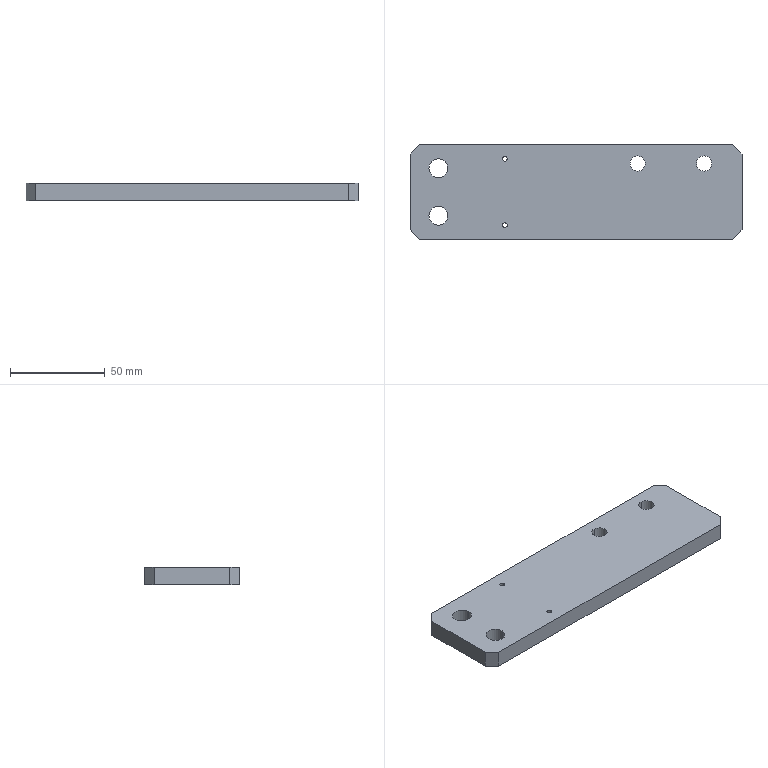Part | STEP file | J013-EBZ05-26-06-Part-1 | 1 solid | 22 faces | box 175 x 50 x 9 mm | volume 75893 mm3 | cylinder 12 | plane 10 | commonest cylinder face diameters 2.5 x4 8 x4 10 x4
STEP:
#1=CARTESIAN_POINT('',(51.25,42.5,9.));
#2=VERTEX_POINT('',#1);
#3=CARTESIAN_POINT('',(48.75,42.5,9.));
#4=VERTEX_POINT('',#3);
#5=CARTESIAN_POINT('',(50.,42.5,9.));
#6=DIRECTION('',(0.,0.,-1.));
#7=DIRECTION('',(-1.,0.,0.));
#8=AXIS2_PLACEMENT_3D('',#5,#6,#7);
#9=CIRCLE('',#8,1.25);
#10=EDGE_CURVE('',#2,#4,#9,.T.);
#11=ORIENTED_EDGE('',*,*,#10,.F.);
#12=CARTESIAN_POINT('',(51.25,42.5,0.));
#13=VERTEX_POINT('',#12);
#14=CARTESIAN_POINT('',(51.25,42.5,9.));
#15=DIRECTION('',(0.,0.,-1.));
#16=VECTOR('',#15,1000.);
#17=LINE('',#14,#16);
#18=EDGE_CURVE('',#2,#13,#17,.T.);
#19=ORIENTED_EDGE('',*,*,#18,.T.);
#20=CARTESIAN_POINT('',(48.75,42.5,0.));
#21=VERTEX_POINT('',#20);
#22=CARTESIAN_POINT('',(50.,42.5,0.));
#23=DIRECTION('',(0.,0.,1.));
#24=DIRECTION('',(1.,0.,0.));
#25=AXIS2_PLACEMENT_3D('',#22,#23,#24);
#26=CIRCLE('',#25,1.25);
#27=EDGE_CURVE('',#21,#13,#26,.T.);
#28=ORIENTED_EDGE('',*,*,#27,.F.);
#29=CARTESIAN_POINT('',(48.75,42.5,9.));
#30=DIRECTION('',(0.,0.,-1.));
#31=VECTOR('',#30,1000.);
#32=LINE('',#29,#31);
#33=EDGE_CURVE('',#4,#21,#32,.T.);
#34=ORIENTED_EDGE('',*,*,#33,.F.);
#35=EDGE_LOOP('',(#11,#19,#28,#34));
#36=FACE_OUTER_BOUND('',#35,.T.);
#37=CARTESIAN_POINT('',(50.,42.5,9.));
#38=DIRECTION('',(0.,0.,-1.));
#39=DIRECTION('',(-1.,0.,0.));
#40=AXIS2_PLACEMENT_3D('',#37,#38,#39);
#41=CYLINDRICAL_SURFACE('',#40,1.25);
#42=ADVANCED_FACE('',(#36),#41,.F.);
#43=CARTESIAN_POINT('',(50.,6.25,9.));
#44=VERTEX_POINT('',#43);
#45=CARTESIAN_POINT('',(50.,8.75,9.));
#46=VERTEX_POINT('',#45);
#47=CARTESIAN_POINT('',(50.,7.5,9.));
#48=DIRECTION('',(0.,0.,-1.));
#49=DIRECTION('',(0.,1.,0.));
#50=AXIS2_PLACEMENT_3D('',#47,#48,#49);
#51=CIRCLE('',#50,1.25);
#52=EDGE_CURVE('',#44,#46,#51,.T.);
#53=ORIENTED_EDGE('',*,*,#52,.F.);
#54=CARTESIAN_POINT('',(50.,6.25,0.));
#55=VERTEX_POINT('',#54);
#56=CARTESIAN_POINT('',(50.,6.25,9.));
#57=DIRECTION('',(0.,0.,-1.));
#58=VECTOR('',#57,1000.);
#59=LINE('',#56,#58);
#60=EDGE_CURVE('',#44,#55,#59,.T.);
#61=ORIENTED_EDGE('',*,*,#60,.T.);
#62=CARTESIAN_POINT('',(50.,8.75,0.));
#63=VERTEX_POINT('',#62);
#64=CARTESIAN_POINT('',(50.,7.5,0.));
#65=DIRECTION('',(0.,0.,1.));
#66=DIRECTION('',(0.,-1.,0.));
#67=AXIS2_PLACEMENT_3D('',#64,#65,#66);
#68=CIRCLE('',#67,1.25);
#69=EDGE_CURVE('',#63,#55,#68,.T.);
#70=ORIENTED_EDGE('',*,*,#69,.F.);
#71=CARTESIAN_POINT('',(50.,8.75,9.));
#72=DIRECTION('',(0.,0.,-1.));
#73=VECTOR('',#72,1000.);
#74=LINE('',#71,#73);
#75=EDGE_CURVE('',#46,#63,#74,.T.);
#76=ORIENTED_EDGE('',*,*,#75,.F.);
#77=EDGE_LOOP('',(#53,#61,#70,#76));
#78=FACE_OUTER_BOUND('',#77,.T.);
#79=CARTESIAN_POINT('',(50.,7.5,9.));
#80=DIRECTION('',(0.,0.,-1.));
#81=DIRECTION('',(0.,1.,0.));
#82=AXIS2_PLACEMENT_3D('',#79,#80,#81);
#83=CYLINDRICAL_SURFACE('',#82,1.25);
#84=ADVANCED_FACE('',(#78),#83,.F.);
#85=CARTESIAN_POINT('',(155.,36.,9.));
#86=VERTEX_POINT('',#85);
#87=CARTESIAN_POINT('',(155.,44.,9.));
#88=VERTEX_POINT('',#87);
#89=CARTESIAN_POINT('',(155.,40.,9.));
#90=DIRECTION('',(0.,0.,-1.));
#91=DIRECTION('',(0.,1.,0.));
#92=AXIS2_PLACEMENT_3D('',#89,#90,#91);
#93=CIRCLE('',#92,4.);
#94=EDGE_CURVE('',#86,#88,#93,.T.);
#95=ORIENTED_EDGE('',*,*,#94,.F.);
#96=CARTESIAN_POINT('',(155.,36.,0.));
#97=VERTEX_POINT('',#96);
#98=CARTESIAN_POINT('',(155.,36.,9.));
#99=DIRECTION('',(0.,0.,-1.));
#100=VECTOR('',#99,1000.);
#101=LINE('',#98,#100);
#102=EDGE_CURVE('',#86,#97,#101,.T.);
#103=ORIENTED_EDGE('',*,*,#102,.T.);
#104=CARTESIAN_POINT('',(155.,44.,0.));
#105=VERTEX_POINT('',#104);
#106=CARTESIAN_POINT('',(155.,40.,0.));
#107=DIRECTION('',(0.,0.,1.));
#108=DIRECTION('',(0.,-1.,0.));
#109=AXIS2_PLACEMENT_3D('',#106,#107,#108);
#110=CIRCLE('',#109,4.);
#111=EDGE_CURVE('',#105,#97,#110,.T.);
#112=ORIENTED_EDGE('',*,*,#111,.F.);
#113=CARTESIAN_POINT('',(155.,44.,9.));
#114=DIRECTION('',(0.,0.,-1.));
#115=VECTOR('',#114,1000.);
#116=LINE('',#113,#115);
#117=EDGE_CURVE('',#88,#105,#116,.T.);
#118=ORIENTED_EDGE('',*,*,#117,.F.);
#119=EDGE_LOOP('',(#95,#103,#112,#118));
#120=FACE_OUTER_BOUND('',#119,.T.);
#121=CARTESIAN_POINT('',(155.,40.,9.));
#122=DIRECTION('',(0.,0.,-1.));
#123=DIRECTION('',(0.,1.,0.));
#124=AXIS2_PLACEMENT_3D('',#121,#122,#123);
#125=CYLINDRICAL_SURFACE('',#124,4.);
#126=ADVANCED_FACE('',(#120),#125,.F.);
#127=CARTESIAN_POINT('',(120.,36.,9.));
#128=VERTEX_POINT('',#127);
#129=CARTESIAN_POINT('',(120.,44.,9.));
#130=VERTEX_POINT('',#129);
#131=CARTESIAN_POINT('',(120.,40.,9.));
#132=DIRECTION('',(0.,0.,-1.));
#133=DIRECTION('',(0.,1.,0.));
#134=AXIS2_PLACEMENT_3D('',#131,#132,#133);
#135=CIRCLE('',#134,4.);
#136=EDGE_CURVE('',#128,#130,#135,.T.);
#137=ORIENTED_EDGE('',*,*,#136,.F.);
#138=CARTESIAN_POINT('',(120.,36.,0.));
#139=VERTEX_POINT('',#138);
#140=CARTESIAN_POINT('',(120.,36.,9.));
#141=DIRECTION('',(0.,0.,-1.));
#142=VECTOR('',#141,1000.);
#143=LINE('',#140,#142);
#144=EDGE_CURVE('',#128,#139,#143,.T.);
#145=ORIENTED_EDGE('',*,*,#144,.T.);
#146=CARTESIAN_POINT('',(120.,44.,0.));
#147=VERTEX_POINT('',#146);
#148=CARTESIAN_POINT('',(120.,40.,0.));
#149=DIRECTION('',(0.,0.,1.));
#150=DIRECTION('',(0.,-1.,0.));
#151=AXIS2_PLACEMENT_3D('',#148,#149,#150);
#152=CIRCLE('',#151,4.);
#153=EDGE_CURVE('',#147,#139,#152,.T.);
#154=ORIENTED_EDGE('',*,*,#153,.F.);
#155=CARTESIAN_POINT('',(120.,44.,9.));
#156=DIRECTION('',(0.,0.,-1.));
#157=VECTOR('',#156,1000.);
#158=LINE('',#155,#157);
#159=EDGE_CURVE('',#130,#147,#158,.T.);
#160=ORIENTED_EDGE('',*,*,#159,.F.);
#161=EDGE_LOOP('',(#137,#145,#154,#160));
#162=FACE_OUTER_BOUND('',#161,.T.);
#163=CARTESIAN_POINT('',(120.,40.,9.));
#164=DIRECTION('',(0.,0.,-1.));
#165=DIRECTION('',(0.,1.,0.));
#166=AXIS2_PLACEMENT_3D('',#163,#164,#165);
#167=CYLINDRICAL_SURFACE('',#166,4.);
#168=ADVANCED_FACE('',(#162),#167,.F.);
#169=CARTESIAN_POINT('',(20.,37.5,9.));
#170=VERTEX_POINT('',#169);
#171=CARTESIAN_POINT('',(10.,37.5,9.));
#172=VERTEX_POINT('',#171);
#173=CARTESIAN_POINT('',(15.,37.5,9.));
#174=DIRECTION('',(0.,0.,-1.));
#175=DIRECTION('',(-1.,0.,0.));
#176=AXIS2_PLACEMENT_3D('',#173,#174,#175);
#177=CIRCLE('',#176,5.);
#178=EDGE_CURVE('',#170,#172,#177,.T.);
#179=ORIENTED_EDGE('',*,*,#178,.F.);
#180=CARTESIAN_POINT('',(20.,37.5,0.));
#181=VERTEX_POINT('',#180);
#182=CARTESIAN_POINT('',(20.,37.5,9.));
#183=DIRECTION('',(0.,0.,-1.));
#184=VECTOR('',#183,1000.);
#185=LINE('',#182,#184);
#186=EDGE_CURVE('',#170,#181,#185,.T.);
#187=ORIENTED_EDGE('',*,*,#186,.T.);
#188=CARTESIAN_POINT('',(10.,37.5,0.));
#189=VERTEX_POINT('',#188);
#190=CARTESIAN_POINT('',(15.,37.5,0.));
#191=DIRECTION('',(0.,0.,1.));
#192=DIRECTION('',(1.,0.,0.));
#193=AXIS2_PLACEMENT_3D('',#190,#191,#192);
#194=CIRCLE('',#193,5.);
#195=EDGE_CURVE('',#189,#181,#194,.T.);
#196=ORIENTED_EDGE('',*,*,#195,.F.);
#197=CARTESIAN_POINT('',(10.,37.5,9.));
#198=DIRECTION('',(0.,0.,-1.));
#199=VECTOR('',#198,1000.);
#200=LINE('',#197,#199);
#201=EDGE_CURVE('',#172,#189,#200,.T.);
#202=ORIENTED_EDGE('',*,*,#201,.F.);
#203=EDGE_LOOP('',(#179,#187,#196,#202));
#204=FACE_OUTER_BOUND('',#203,.T.);
#205=CARTESIAN_POINT('',(15.,37.5,9.));
#206=DIRECTION('',(0.,0.,-1.));
#207=DIRECTION('',(-1.,0.,0.));
#208=AXIS2_PLACEMENT_3D('',#205,#206,#207);
#209=CYLINDRICAL_SURFACE('',#208,5.);
#210=ADVANCED_FACE('',(#204),#209,.F.);
#211=CARTESIAN_POINT('',(20.,12.5,9.));
#212=VERTEX_POINT('',#211);
#213=CARTESIAN_POINT('',(10.,12.5,9.));
#214=VERTEX_POINT('',#213);
#215=CARTESIAN_POINT('',(15.,12.5,9.));
#216=DIRECTION('',(0.,0.,-1.));
#217=DIRECTION('',(-1.,0.,0.));
#218=AXIS2_PLACEMENT_3D('',#215,#216,#217);
#219=CIRCLE('',#218,5.);
#220=EDGE_CURVE('',#212,#214,#219,.T.);
#221=ORIENTED_EDGE('',*,*,#220,.F.);
#222=CARTESIAN_POINT('',(20.,12.5,0.));
#223=VERTEX_POINT('',#222);
#224=CARTESIAN_POINT('',(20.,12.5,9.));
#225=DIRECTION('',(0.,0.,-1.));
#226=VECTOR('',#225,1000.);
#227=LINE('',#224,#226);
#228=EDGE_CURVE('',#212,#223,#227,.T.);
#229=ORIENTED_EDGE('',*,*,#228,.T.);
#230=CARTESIAN_POINT('',(10.,12.5,0.));
#231=VERTEX_POINT('',#230);
#232=CARTESIAN_POINT('',(15.,12.5,0.));
#233=DIRECTION('',(0.,0.,1.));
#234=DIRECTION('',(1.,0.,0.));
#235=AXIS2_PLACEMENT_3D('',#232,#233,#234);
#236=CIRCLE('',#235,5.);
#237=EDGE_CURVE('',#231,#223,#236,.T.);
#238=ORIENTED_EDGE('',*,*,#237,.F.);
#239=CARTESIAN_POINT('',(10.,12.5,9.));
#240=DIRECTION('',(0.,0.,-1.));
#241=VECTOR('',#240,1000.);
#242=LINE('',#239,#241);
#243=EDGE_CURVE('',#214,#231,#242,.T.);
#244=ORIENTED_EDGE('',*,*,#243,.F.);
#245=EDGE_LOOP('',(#221,#229,#238,#244));
#246=FACE_OUTER_BOUND('',#245,.T.);
#247=CARTESIAN_POINT('',(15.,12.5,9.));
#248=DIRECTION('',(0.,0.,-1.));
#249=DIRECTION('',(-1.,0.,0.));
#250=AXIS2_PLACEMENT_3D('',#247,#248,#249);
#251=CYLINDRICAL_SURFACE('',#250,5.);
#252=ADVANCED_FACE('',(#246),#251,.F.);
#253=ORIENTED_EDGE('',*,*,#27,.T.);
#254=CARTESIAN_POINT('',(50.,42.5,0.));
#255=DIRECTION('',(0.,0.,1.));
#256=DIRECTION('',(1.,0.,0.));
#257=AXIS2_PLACEMENT_3D('',#254,#255,#256);
#258=CIRCLE('',#257,1.25);
#259=EDGE_CURVE('',#13,#21,#258,.T.);
#260=ORIENTED_EDGE('',*,*,#259,.T.);
#261=EDGE_LOOP('',(#253,#260));
#262=FACE_BOUND('',#261,.T.);
#263=ORIENTED_EDGE('',*,*,#69,.T.);
#264=CARTESIAN_POINT('',(50.,7.5,0.));
#265=DIRECTION('',(0.,0.,1.));
#266=DIRECTION('',(0.,-1.,0.));
#267=AXIS2_PLACEMENT_3D('',#264,#265,#266);
#268=CIRCLE('',#267,1.25);
#269=EDGE_CURVE('',#55,#63,#268,.T.);
#270=ORIENTED_EDGE('',*,*,#269,.T.);
#271=EDGE_LOOP('',(#263,#270));
#272=FACE_BOUND('',#271,.T.);
#273=ORIENTED_EDGE('',*,*,#111,.T.);
#274=CARTESIAN_POINT('',(155.,40.,0.));
#275=DIRECTION('',(0.,0.,1.));
#276=DIRECTION('',(0.,-1.,0.));
#277=AXIS2_PLACEMENT_3D('',#274,#275,#276);
#278=CIRCLE('',#277,4.);
#279=EDGE_CURVE('',#97,#105,#278,.T.);
#280=ORIENTED_EDGE('',*,*,#279,.T.);
#281=EDGE_LOOP('',(#273,#280));
#282=FACE_BOUND('',#281,.T.);
#283=ORIENTED_EDGE('',*,*,#153,.T.);
#284=CARTESIAN_POINT('',(120.,40.,0.));
#285=DIRECTION('',(0.,0.,1.));
#286=DIRECTION('',(0.,-1.,0.));
#287=AXIS2_PLACEMENT_3D('',#284,#285,#286);
#288=CIRCLE('',#287,4.);
#289=EDGE_CURVE('',#139,#147,#288,.T.);
#290=ORIENTED_EDGE('',*,*,#289,.T.);
#291=EDGE_LOOP('',(#283,#290));
#292=FACE_BOUND('',#291,.T.);
#293=ORIENTED_EDGE('',*,*,#195,.T.);
#294=CARTESIAN_POINT('',(15.,37.5,0.));
#295=DIRECTION('',(0.,0.,1.));
#296=DIRECTION('',(1.,0.,0.));
#297=AXIS2_PLACEMENT_3D('',#294,#295,#296);
#298=CIRCLE('',#297,5.);
#299=EDGE_CURVE('',#181,#189,#298,.T.);
#300=ORIENTED_EDGE('',*,*,#299,.T.);
#301=EDGE_LOOP('',(#293,#300));
#302=FACE_BOUND('',#301,.T.);
#303=ORIENTED_EDGE('',*,*,#237,.T.);
#304=CARTESIAN_POINT('',(15.,12.5,0.));
#305=DIRECTION('',(0.,0.,1.));
#306=DIRECTION('',(1.,0.,0.));
#307=AXIS2_PLACEMENT_3D('',#304,#305,#306);
#308=CIRCLE('',#307,5.);
#309=EDGE_CURVE('',#223,#231,#308,.T.);
#310=ORIENTED_EDGE('',*,*,#309,.T.);
#311=EDGE_LOOP('',(#303,#310));
#312=FACE_BOUND('',#311,.T.);
#313=CARTESIAN_POINT('',(170.,50.,0.));
#314=VERTEX_POINT('',#313);
#315=CARTESIAN_POINT('',(5.,50.,0.));
#316=VERTEX_POINT('',#315);
#317=CARTESIAN_POINT('',(87.5,50.,0.));
#318=DIRECTION('',(-1.,0.,0.));
#319=VECTOR('',#318,1000.);
#320=LINE('',#317,#319);
#321=EDGE_CURVE('',#314,#316,#320,.T.);
#322=ORIENTED_EDGE('',*,*,#321,.F.);
#323=CARTESIAN_POINT('',(175.,45.,0.));
#324=VERTEX_POINT('',#323);
#325=CARTESIAN_POINT('',(141.25,78.75,0.));
#326=DIRECTION('',(0.7071,-0.7071,0.));
#327=VECTOR('',#326,1000.);
#328=LINE('',#325,#327);
#329=EDGE_CURVE('',#314,#324,#328,.T.);
#330=ORIENTED_EDGE('',*,*,#329,.T.);
#331=CARTESIAN_POINT('',(175.,5.,0.));
#332=VERTEX_POINT('',#331);
#333=CARTESIAN_POINT('',(175.,25.,0.));
#334=DIRECTION('',(0.,1.,0.));
#335=VECTOR('',#334,1000.);
#336=LINE('',#333,#335);
#337=EDGE_CURVE('',#332,#324,#336,.T.);
#338=ORIENTED_EDGE('',*,*,#337,.F.);
#339=CARTESIAN_POINT('',(170.,0.,0.));
#340=VERTEX_POINT('',#339);
#341=CARTESIAN_POINT('',(141.25,-28.75,0.));
#342=DIRECTION('',(-0.7071,-0.7071,0.));
#343=VECTOR('',#342,1000.);
#344=LINE('',#341,#343);
#345=EDGE_CURVE('',#332,#340,#344,.T.);
#346=ORIENTED_EDGE('',*,*,#345,.T.);
#347=CARTESIAN_POINT('',(5.,0.,0.));
#348=VERTEX_POINT('',#347);
#349=CARTESIAN_POINT('',(87.5,0.,0.));
#350=DIRECTION('',(1.,0.,0.));
#351=VECTOR('',#350,1000.);
#352=LINE('',#349,#351);
#353=EDGE_CURVE('',#348,#340,#352,.T.);
#354=ORIENTED_EDGE('',*,*,#353,.F.);
#355=CARTESIAN_POINT('',(0.,5.,0.));
#356=VERTEX_POINT('',#355);
#357=CARTESIAN_POINT('',(33.75,-28.75,0.));
#358=DIRECTION('',(-0.7071,0.7071,0.));
#359=VECTOR('',#358,1000.);
#360=LINE('',#357,#359);
#361=EDGE_CURVE('',#348,#356,#360,.T.);
#362=ORIENTED_EDGE('',*,*,#361,.T.);
#363=CARTESIAN_POINT('',(0.,45.,0.));
#364=VERTEX_POINT('',#363);
#365=CARTESIAN_POINT('',(0.,25.,0.));
#366=DIRECTION('',(0.,-1.,0.));
#367=VECTOR('',#366,1000.);
#368=LINE('',#365,#367);
#369=EDGE_CURVE('',#364,#356,#368,.T.);
#370=ORIENTED_EDGE('',*,*,#369,.F.);
#371=CARTESIAN_POINT('',(33.75,78.75,0.));
#372=DIRECTION('',(0.7071,0.7071,0.));
#373=VECTOR('',#372,1000.);
#374=LINE('',#371,#373);
#375=EDGE_CURVE('',#364,#316,#374,.T.);
#376=ORIENTED_EDGE('',*,*,#375,.T.);
#377=EDGE_LOOP('',(#322,#330,#338,#346,#354,#362,#370,#376));
#378=FACE_OUTER_BOUND('',#377,.T.);
#379=CARTESIAN_POINT('',(87.5,25.,0.));
#380=DIRECTION('',(0.,0.,-1.));
#381=DIRECTION('',(0.,1.,0.));
#382=AXIS2_PLACEMENT_3D('',#379,#380,#381);
#383=PLANE('',#382);
#384=ADVANCED_FACE('',(#262,#272,#282,#292,#302,#312,#378),#383,.T.);
#385=CARTESIAN_POINT('',(0.,5.,9.));
#386=VERTEX_POINT('',#385);
#387=CARTESIAN_POINT('',(0.,45.,9.));
#388=VERTEX_POINT('',#387);
#389=CARTESIAN_POINT('',(0.,25.,9.));
#390=DIRECTION('',(0.,1.,0.));
#391=VECTOR('',#390,1000.);
#392=LINE('',#389,#391);
#393=EDGE_CURVE('',#386,#388,#392,.T.);
#394=ORIENTED_EDGE('',*,*,#393,.T.);
#395=CARTESIAN_POINT('',(0.,45.,9.));
#396=DIRECTION('',(0.,0.,-1.));
#397=VECTOR('',#396,1000.);
#398=LINE('',#395,#397);
#399=EDGE_CURVE('',#388,#364,#398,.T.);
#400=ORIENTED_EDGE('',*,*,#399,.T.);
#401=ORIENTED_EDGE('',*,*,#369,.T.);
#402=CARTESIAN_POINT('',(0.,5.,9.));
#403=DIRECTION('',(0.,0.,1.));
#404=VECTOR('',#403,1000.);
#405=LINE('',#402,#404);
#406=EDGE_CURVE('',#356,#386,#405,.T.);
#407=ORIENTED_EDGE('',*,*,#406,.T.);
#408=EDGE_LOOP('',(#394,#400,#401,#407));
#409=FACE_OUTER_BOUND('',#408,.T.);
#410=CARTESIAN_POINT('',(0.,25.,9.));
#411=DIRECTION('',(-1.,0.,0.));
#412=DIRECTION('',(0.,0.,1.));
#413=AXIS2_PLACEMENT_3D('',#410,#411,#412);
#414=PLANE('',#413);
#415=ADVANCED_FACE('',(#409),#414,.T.);
#416=ORIENTED_EDGE('',*,*,#353,.T.);
#417=CARTESIAN_POINT('',(170.,0.,9.));
#418=VERTEX_POINT('',#417);
#419=CARTESIAN_POINT('',(170.,0.,9.));
#420=DIRECTION('',(0.,0.,1.));
#421=VECTOR('',#420,1000.);
#422=LINE('',#419,#421);
#423=EDGE_CURVE('',#340,#418,#422,.T.);
#424=ORIENTED_EDGE('',*,*,#423,.T.);
#425=CARTESIAN_POINT('',(5.,0.,9.));
#426=VERTEX_POINT('',#425);
#427=CARTESIAN_POINT('',(87.5,0.,9.));
#428=DIRECTION('',(-1.,0.,0.));
#429=VECTOR('',#428,1000.);
#430=LINE('',#427,#429);
#431=EDGE_CURVE('',#418,#426,#430,.T.);
#432=ORIENTED_EDGE('',*,*,#431,.T.);
#433=CARTESIAN_POINT('',(5.,0.,9.));
#434=DIRECTION('',(0.,0.,-1.));
#435=VECTOR('',#434,1000.);
#436=LINE('',#433,#435);
#437=EDGE_CURVE('',#426,#348,#436,.T.);
#438=ORIENTED_EDGE('',*,*,#437,.T.);
#439=EDGE_LOOP('',(#416,#424,#432,#438));
#440=FACE_OUTER_BOUND('',#439,.T.);
#441=CARTESIAN_POINT('',(87.5,0.,9.));
#442=DIRECTION('',(0.,-1.,0.));
#443=DIRECTION('',(0.,0.,-1.));
#444=AXIS2_PLACEMENT_3D('',#441,#442,#443);
#445=PLANE('',#444);
#446=ADVANCED_FACE('',(#440),#445,.T.);
#447=ORIENTED_EDGE('',*,*,#337,.T.);
#448=CARTESIAN_POINT('',(175.,45.,9.));
#449=VERTEX_POINT('',#448);
#450=CARTESIAN_POINT('',(175.,45.,9.));
#451=DIRECTION('',(0.,0.,1.));
#452=VECTOR('',#451,1000.);
#453=LINE('',#450,#452);
#454=EDGE_CURVE('',#324,#449,#453,.T.);
#455=ORIENTED_EDGE('',*,*,#454,.T.);
#456=CARTESIAN_POINT('',(175.,5.,9.));
#457=VERTEX_POINT('',#456);
#458=CARTESIAN_POINT('',(175.,25.,9.));
#459=DIRECTION('',(0.,-1.,0.));
#460=VECTOR('',#459,1000.);
#461=LINE('',#458,#460);
#462=EDGE_CURVE('',#449,#457,#461,.T.);
#463=ORIENTED_EDGE('',*,*,#462,.T.);
#464=CARTESIAN_POINT('',(175.,5.,9.));
#465=DIRECTION('',(0.,0.,-1.));
#466=VECTOR('',#465,1000.);
#467=LINE('',#464,#466);
#468=EDGE_CURVE('',#457,#332,#467,.T.);
#469=ORIENTED_EDGE('',*,*,#468,.T.);
#470=EDGE_LOOP('',(#447,#455,#463,#469));
#471=FACE_OUTER_BOUND('',#470,.T.);
#472=CARTESIAN_POINT('',(175.,25.,9.));
#473=DIRECTION('',(1.,0.,0.));
#474=DIRECTION('',(0.,0.,-1.));
#475=AXIS2_PLACEMENT_3D('',#472,#473,#474);
#476=PLANE('',#475);
#477=ADVANCED_FACE('',(#471),#476,.T.);
#478=CARTESIAN_POINT('',(50.,42.5,9.));
#479=DIRECTION('',(0.,0.,-1.));
#480=DIRECTION('',(-1.,0.,0.));
#481=AXIS2_PLACEMENT_3D('',#478,#479,#480);
#482=CIRCLE('',#481,1.25);
#483=EDGE_CURVE('',#4,#2,#482,.T.);
#484=ORIENTED_EDGE('',*,*,#483,.T.);
#485=ORIENTED_EDGE('',*,*,#10,.T.);
#486=EDGE_LOOP('',(#484,#485));
#487=FACE_BOUND('',#486,.T.);
#488=CARTESIAN_POINT('',(50.,7.5,9.));
#489=DIRECTION('',(0.,0.,-1.));
#490=DIRECTION('',(0.,1.,0.));
#491=AXIS2_PLACEMENT_3D('',#488,#489,#490);
#492=CIRCLE('',#491,1.25);
#493=EDGE_CURVE('',#46,#44,#492,.T.);
#494=ORIENTED_EDGE('',*,*,#493,.T.);
#495=ORIENTED_EDGE('',*,*,#52,.T.);
#496=EDGE_LOOP('',(#494,#495));
#497=FACE_BOUND('',#496,.T.);
#498=CARTESIAN_POINT('',(155.,40.,9.));
#499=DIRECTION('',(0.,0.,-1.));
#500=DIRECTION('',(0.,1.,0.));
#501=AXIS2_PLACEMENT_3D('',#498,#499,#500);
#502=CIRCLE('',#501,4.);
#503=EDGE_CURVE('',#88,#86,#502,.T.);
#504=ORIENTED_EDGE('',*,*,#503,.T.);
#505=ORIENTED_EDGE('',*,*,#94,.T.);
#506=EDGE_LOOP('',(#504,#505));
#507=FACE_BOUND('',#506,.T.);
#508=CARTESIAN_POINT('',(120.,40.,9.));
#509=DIRECTION('',(0.,0.,-1.));
#510=DIRECTION('',(0.,1.,0.));
#511=AXIS2_PLACEMENT_3D('',#508,#509,#510);
#512=CIRCLE('',#511,4.);
#513=EDGE_CURVE('',#130,#128,#512,.T.);
#514=ORIENTED_EDGE('',*,*,#513,.T.);
#515=ORIENTED_EDGE('',*,*,#136,.T.);
#516=EDGE_LOOP('',(#514,#515));
#517=FACE_BOUND('',#516,.T.);
#518=CARTESIAN_POINT('',(15.,37.5,9.));
#519=DIRECTION('',(0.,0.,-1.));
#520=DIRECTION('',(-1.,0.,0.));
#521=AXIS2_PLACEMENT_3D('',#518,#519,#520);
#522=CIRCLE('',#521,5.);
#523=EDGE_CURVE('',#172,#170,#522,.T.);
#524=ORIENTED_EDGE('',*,*,#523,.T.);
#525=ORIENTED_EDGE('',*,*,#178,.T.);
#526=EDGE_LOOP('',(#524,#525));
#527=FACE_BOUND('',#526,.T.);
#528=CARTESIAN_POINT('',(15.,12.5,9.));
#529=DIRECTION('',(0.,0.,-1.));
#530=DIRECTION('',(-1.,0.,0.));
#531=AXIS2_PLACEMENT_3D('',#528,#529,#530);
#532=CIRCLE('',#531,5.);
#533=EDGE_CURVE('',#214,#212,#532,.T.);
#534=ORIENTED_EDGE('',*,*,#533,.T.);
#535=ORIENTED_EDGE('',*,*,#220,.T.);
#536=EDGE_LOOP('',(#534,#535));
#537=FACE_BOUND('',#536,.T.);
#538=ORIENTED_EDGE('',*,*,#462,.F.);
#539=CARTESIAN_POINT('',(170.,50.,9.));
#540=VERTEX_POINT('',#539);
#541=CARTESIAN_POINT('',(141.25,78.75,9.));
#542=DIRECTION('',(-0.7071,0.7071,0.));
#543=VECTOR('',#542,1000.);
#544=LINE('',#541,#543);
#545=EDGE_CURVE('',#449,#540,#544,.T.);
#546=ORIENTED_EDGE('',*,*,#545,.T.);
#547=CARTESIAN_POINT('',(5.,50.,9.));
#548=VERTEX_POINT('',#547);
#549=CARTESIAN_POINT('',(87.5,50.,9.));
#550=DIRECTION('',(1.,0.,0.));
#551=VECTOR('',#550,1000.);
#552=LINE('',#549,#551);
#553=EDGE_CURVE('',#548,#540,#552,.T.);
#554=ORIENTED_EDGE('',*,*,#553,.F.);
#555=CARTESIAN_POINT('',(33.75,78.75,9.));
#556=DIRECTION('',(-0.7071,-0.7071,0.));
#557=VECTOR('',#556,1000.);
#558=LINE('',#555,#557);
#559=EDGE_CURVE('',#548,#388,#558,.T.);
#560=ORIENTED_EDGE('',*,*,#559,.T.);
#561=ORIENTED_EDGE('',*,*,#393,.F.);
#562=CARTESIAN_POINT('',(33.75,-28.75,9.));
#563=DIRECTION('',(0.7071,-0.7071,0.));
#564=VECTOR('',#563,1000.);
#565=LINE('',#562,#564);
#566=EDGE_CURVE('',#386,#426,#565,.T.);
#567=ORIENTED_EDGE('',*,*,#566,.T.);
#568=ORIENTED_EDGE('',*,*,#431,.F.);
#569=CARTESIAN_POINT('',(141.25,-28.75,9.));
#570=DIRECTION('',(0.7071,0.7071,0.));
#571=VECTOR('',#570,1000.);
#572=LINE('',#569,#571);
#573=EDGE_CURVE('',#418,#457,#572,.T.);
#574=ORIENTED_EDGE('',*,*,#573,.T.);
#575=EDGE_LOOP('',(#538,#546,#554,#560,#561,#567,#568,#574));
#576=FACE_OUTER_BOUND('',#575,.T.);
#577=CARTESIAN_POINT('',(87.5,25.,9.));
#578=DIRECTION('',(0.,0.,1.));
#579=DIRECTION('',(0.,-1.,0.));
#580=AXIS2_PLACEMENT_3D('',#577,#578,#579);
#581=PLANE('',#580);
#582=ADVANCED_FACE('',(#487,#497,#507,#517,#527,#537,#576),#581,.T.);
#583=ORIENTED_EDGE('',*,*,#553,.T.);
#584=CARTESIAN_POINT('',(170.,50.,9.));
#585=DIRECTION('',(0.,0.,-1.));
#586=VECTOR('',#585,1000.);
#587=LINE('',#584,#586);
#588=EDGE_CURVE('',#540,#314,#587,.T.);
#589=ORIENTED_EDGE('',*,*,#588,.T.);
#590=ORIENTED_EDGE('',*,*,#321,.T.);
#591=CARTESIAN_POINT('',(5.,50.,9.));
#592=DIRECTION('',(0.,0.,1.));
#593=VECTOR('',#592,1000.);
#594=LINE('',#591,#593);
#595=EDGE_CURVE('',#316,#548,#594,.T.);
#596=ORIENTED_EDGE('',*,*,#595,.T.);
#597=EDGE_LOOP('',(#583,#589,#590,#596));
#598=FACE_OUTER_BOUND('',#597,.T.);
#599=CARTESIAN_POINT('',(87.5,50.,9.));
#600=DIRECTION('',(0.,1.,0.));
#601=DIRECTION('',(0.,0.,1.));
#602=AXIS2_PLACEMENT_3D('',#599,#600,#601);
#603=PLANE('',#602);
#604=ADVANCED_FACE('',(#598),#603,.T.);
#605=ORIENTED_EDGE('',*,*,#228,.F.);
#606=ORIENTED_EDGE('',*,*,#533,.F.);
#607=ORIENTED_EDGE('',*,*,#243,.T.);
#608=ORIENTED_EDGE('',*,*,#309,.F.);
#609=EDGE_LOOP('',(#605,#606,#607,#608));
#610=FACE_OUTER_BOUND('',#609,.T.);
#611=CARTESIAN_POINT('',(15.,12.5,9.));
#612=DIRECTION('',(0.,0.,-1.));
#613=DIRECTION('',(-1.,0.,0.));
#614=AXIS2_PLACEMENT_3D('',#611,#612,#613);
#615=CYLINDRICAL_SURFACE('',#614,5.);
#616=ADVANCED_FACE('',(#610),#615,.F.);
#617=ORIENTED_EDGE('',*,*,#186,.F.);
#618=ORIENTED_EDGE('',*,*,#523,.F.);
#619=ORIENTED_EDGE('',*,*,#201,.T.);
#620=ORIENTED_EDGE('',*,*,#299,.F.);
#621=EDGE_LOOP('',(#617,#618,#619,#620));
#622=FACE_OUTER_BOUND('',#621,.T.);
#623=CARTESIAN_POINT('',(15.,37.5,9.));
#624=DIRECTION('',(0.,0.,-1.));
#625=DIRECTION('',(-1.,0.,0.));
#626=AXIS2_PLACEMENT_3D('',#623,#624,#625);
#627=CYLINDRICAL_SURFACE('',#626,5.);
#628=ADVANCED_FACE('',(#622),#627,.F.);
#629=ORIENTED_EDGE('',*,*,#144,.F.);
#630=ORIENTED_EDGE('',*,*,#513,.F.);
#631=ORIENTED_EDGE('',*,*,#159,.T.);
#632=ORIENTED_EDGE('',*,*,#289,.F.);
#633=EDGE_LOOP('',(#629,#630,#631,#632));
#634=FACE_OUTER_BOUND('',#633,.T.);
#635=CARTESIAN_POINT('',(120.,40.,9.));
#636=DIRECTION('',(0.,0.,-1.));
#637=DIRECTION('',(0.,1.,0.));
#638=AXIS2_PLACEMENT_3D('',#635,#636,#637);
#639=CYLINDRICAL_SURFACE('',#638,4.);
#640=ADVANCED_FACE('',(#634),#639,.F.);
#641=ORIENTED_EDGE('',*,*,#102,.F.);
#642=ORIENTED_EDGE('',*,*,#503,.F.);
#643=ORIENTED_EDGE('',*,*,#117,.T.);
#644=ORIENTED_EDGE('',*,*,#279,.F.);
#645=EDGE_LOOP('',(#641,#642,#643,#644));
#646=FACE_OUTER_BOUND('',#645,.T.);
#647=CARTESIAN_POINT('',(155.,40.,9.));
#648=DIRECTION('',(0.,0.,-1.));
#649=DIRECTION('',(0.,1.,0.));
#650=AXIS2_PLACEMENT_3D('',#647,#648,#649);
#651=CYLINDRICAL_SURFACE('',#650,4.);
#652=ADVANCED_FACE('',(#646),#651,.F.);
#653=ORIENTED_EDGE('',*,*,#566,.F.);
#654=ORIENTED_EDGE('',*,*,#406,.F.);
#655=ORIENTED_EDGE('',*,*,#361,.F.);
#656=ORIENTED_EDGE('',*,*,#437,.F.);
#657=EDGE_LOOP('',(#653,#654,#655,#656));
#658=FACE_OUTER_BOUND('',#657,.T.);
#659=CARTESIAN_POINT('',(5.,0.,9.));
#660=DIRECTION('',(0.7071,0.7071,0.));
#661=DIRECTION('',(0.,0.,-1.));
#662=AXIS2_PLACEMENT_3D('',#659,#660,#661);
#663=PLANE('',#662);
#664=ADVANCED_FACE('',(#658),#663,.F.);
#665=ORIENTED_EDGE('',*,*,#559,.F.);
#666=ORIENTED_EDGE('',*,*,#595,.F.);
#667=ORIENTED_EDGE('',*,*,#375,.F.);
#668=ORIENTED_EDGE('',*,*,#399,.F.);
#669=EDGE_LOOP('',(#665,#666,#667,#668));
#670=FACE_OUTER_BOUND('',#669,.T.);
#671=CARTESIAN_POINT('',(0.,45.,9.));
#672=DIRECTION('',(0.7071,-0.7071,0.));
#673=DIRECTION('',(0.,0.,-1.));
#674=AXIS2_PLACEMENT_3D('',#671,#672,#673);
#675=PLANE('',#674);
#676=ADVANCED_FACE('',(#670),#675,.F.);
#677=ORIENTED_EDGE('',*,*,#573,.F.);
#678=ORIENTED_EDGE('',*,*,#423,.F.);
#679=ORIENTED_EDGE('',*,*,#345,.F.);
#680=ORIENTED_EDGE('',*,*,#468,.F.);
#681=EDGE_LOOP('',(#677,#678,#679,#680));
#682=FACE_OUTER_BOUND('',#681,.T.);
#683=CARTESIAN_POINT('',(175.,5.,9.));
#684=DIRECTION('',(-0.7071,0.7071,0.));
#685=DIRECTION('',(0.,0.,-1.));
#686=AXIS2_PLACEMENT_3D('',#683,#684,#685);
#687=PLANE('',#686);
#688=ADVANCED_FACE('',(#682),#687,.F.);
#689=ORIENTED_EDGE('',*,*,#545,.F.);
#690=ORIENTED_EDGE('',*,*,#454,.F.);
#691=ORIENTED_EDGE('',*,*,#329,.F.);
#692=ORIENTED_EDGE('',*,*,#588,.F.);
#693=EDGE_LOOP('',(#689,#690,#691,#692));
#694=FACE_OUTER_BOUND('',#693,.T.);
#695=CARTESIAN_POINT('',(170.,50.,9.));
#696=DIRECTION('',(-0.7071,-0.7071,0.));
#697=DIRECTION('',(0.,0.,-1.));
#698=AXIS2_PLACEMENT_3D('',#695,#696,#697);
#699=PLANE('',#698);
#700=ADVANCED_FACE('',(#694),#699,.F.);
#701=ORIENTED_EDGE('',*,*,#60,.F.);
#702=ORIENTED_EDGE('',*,*,#493,.F.);
#703=ORIENTED_EDGE('',*,*,#75,.T.);
#704=ORIENTED_EDGE('',*,*,#269,.F.);
#705=EDGE_LOOP('',(#701,#702,#703,#704));
#706=FACE_OUTER_BOUND('',#705,.T.);
#707=CARTESIAN_POINT('',(50.,7.5,9.));
#708=DIRECTION('',(0.,0.,-1.));
#709=DIRECTION('',(0.,1.,0.));
#710=AXIS2_PLACEMENT_3D('',#707,#708,#709);
#711=CYLINDRICAL_SURFACE('',#710,1.25);
#712=ADVANCED_FACE('',(#706),#711,.F.);
#713=ORIENTED_EDGE('',*,*,#18,.F.);
#714=ORIENTED_EDGE('',*,*,#483,.F.);
#715=ORIENTED_EDGE('',*,*,#33,.T.);
#716=ORIENTED_EDGE('',*,*,#259,.F.);
#717=EDGE_LOOP('',(#713,#714,#715,#716));
#718=FACE_OUTER_BOUND('',#717,.T.);
#719=CARTESIAN_POINT('',(50.,42.5,9.));
#720=DIRECTION('',(0.,0.,-1.));
#721=DIRECTION('',(-1.,0.,0.));
#722=AXIS2_PLACEMENT_3D('',#719,#720,#721);
#723=CYLINDRICAL_SURFACE('',#722,1.25);
#724=ADVANCED_FACE('',(#718),#723,.F.);
#725=CLOSED_SHELL('',(#42,#84,#126,#168,#210,#252,#384,#415,#446,#477,#582,#604,#616,#628,#640,#652,#664,#676,#688,#700,#712,#724));
#726=MANIFOLD_SOLID_BREP('',#725);
#727=CARTESIAN_POINT('',(0.,0.,0.));
#728=DIRECTION('',(0.,0.,1.));
#729=DIRECTION('',(1.,0.,0.));
#730=AXIS2_PLACEMENT_3D('',#727,#728,#729);
#731=(LENGTH_UNIT()NAMED_UNIT(*)SI_UNIT(.MILLI.,.METRE.));
#732=UNCERTAINTY_MEASURE_WITH_UNIT(LENGTH_MEASURE(0.00001),#731,'','');
#733=(NAMED_UNIT(*)PLANE_ANGLE_UNIT()SI_UNIT($,.RADIAN.));
#734=(NAMED_UNIT(*)SI_UNIT($,.STERADIAN.)SOLID_ANGLE_UNIT());
#735=(GEOMETRIC_REPRESENTATION_CONTEXT(3)GLOBAL_UNCERTAINTY_ASSIGNED_CONTEXT((#732))GLOBAL_UNIT_ASSIGNED_CONTEXT((#731,#733,#734))REPRESENTATION_CONTEXT('',''));
#736=ADVANCED_BREP_SHAPE_REPRESENTATION('',(#726,#730),#735);